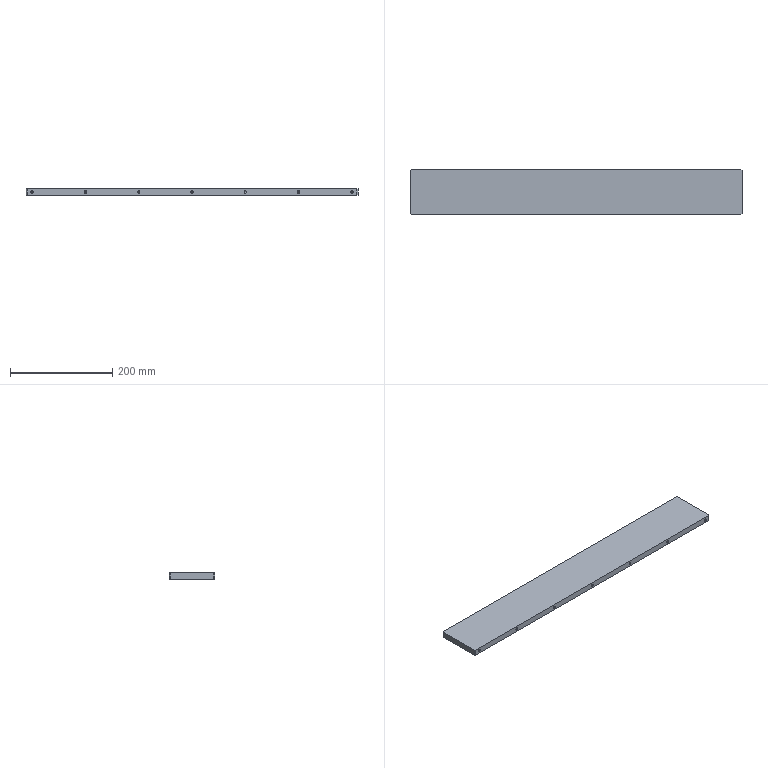Part | STEP file | 001-010-Waste base plate | 1 solid | 38 faces | box 650 x 90 x 12 mm | volume 699774 mm3 | cylinder 14 | cone 14 | plane 10 | commonest cylinder face diameters 5 x14